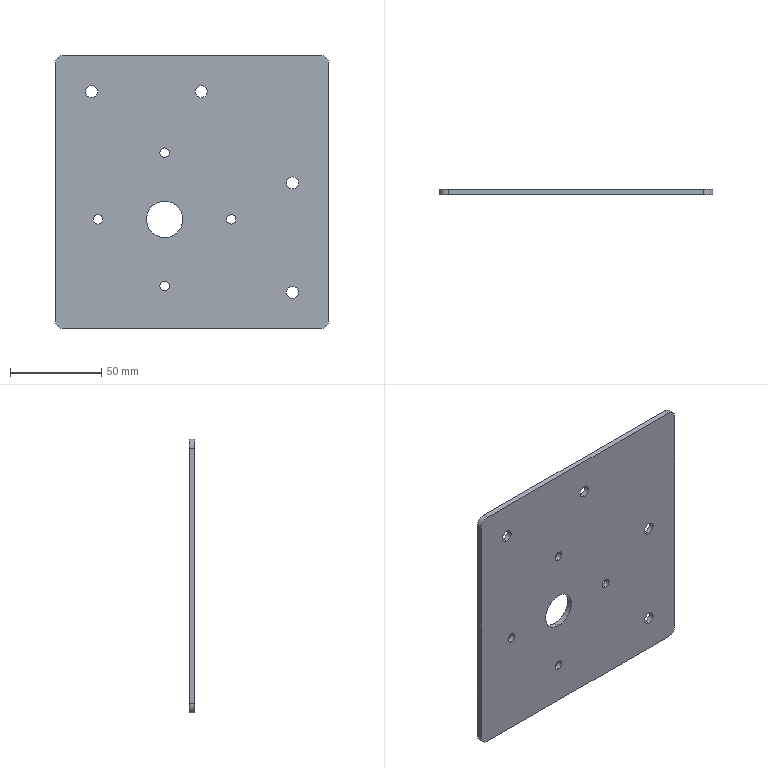Part | SolidWorks | features Extrusion 1, Fillet 1, HoleWzd 1, ICE 1 | 1 solid | 28 faces | box 150 x 3 x 150 mm | volume 65828 mm3 | cylinder 22 | plane 6 | commonest cylinder face diameters 5.2 x8 6.6 x8 10 x4 20 x2
STEP:
#1=CARTESIAN_POINT('',(-51.5,0.,-17.6));
#2=VERTEX_POINT('',#1);
#3=CARTESIAN_POINT('',(-51.5,0.,-12.4));
#4=VERTEX_POINT('',#3);
#5=CARTESIAN_POINT('',(-51.5,0.,-15.));
#6=DIRECTION('',(0.,1.,0.));
#7=DIRECTION('',(0.,0.,1.));
#8=AXIS2_PLACEMENT_3D('',#5,#6,#7);
#9=CIRCLE('',#8,2.6);
#10=EDGE_CURVE('',#2,#4,#9,.T.);
#11=ORIENTED_EDGE('',*,*,#10,.F.);
#12=CARTESIAN_POINT('',(-51.5,3.,-17.6));
#13=VERTEX_POINT('',#12);
#14=CARTESIAN_POINT('',(-51.5,0.,-17.6));
#15=DIRECTION('',(0.,1.,0.));
#16=VECTOR('',#15,1000.);
#17=LINE('',#14,#16);
#18=EDGE_CURVE('',#2,#13,#17,.T.);
#19=ORIENTED_EDGE('',*,*,#18,.T.);
#20=CARTESIAN_POINT('',(-51.5,3.,-12.4));
#21=VERTEX_POINT('',#20);
#22=CARTESIAN_POINT('',(-51.5,3.,-15.));
#23=DIRECTION('',(0.,1.,0.));
#24=DIRECTION('',(0.,0.,1.));
#25=AXIS2_PLACEMENT_3D('',#22,#23,#24);
#26=CIRCLE('',#25,2.6);
#27=EDGE_CURVE('',#13,#21,#26,.T.);
#28=ORIENTED_EDGE('',*,*,#27,.T.);
#29=CARTESIAN_POINT('',(-51.5,0.,-12.4));
#30=DIRECTION('',(0.,1.,0.));
#31=VECTOR('',#30,1000.);
#32=LINE('',#29,#31);
#33=EDGE_CURVE('',#4,#21,#32,.T.);
#34=ORIENTED_EDGE('',*,*,#33,.F.);
#35=EDGE_LOOP('',(#11,#19,#28,#34));
#36=FACE_OUTER_BOUND('',#35,.T.);
#37=CARTESIAN_POINT('',(-51.5,0.,-15.));
#38=DIRECTION('',(0.,1.,0.));
#39=DIRECTION('',(0.,0.,1.));
#40=AXIS2_PLACEMENT_3D('',#37,#38,#39);
#41=CYLINDRICAL_SURFACE('',#40,2.6);
#42=ADVANCED_FACE('',(#36),#41,.F.);
#43=CARTESIAN_POINT('',(-15.,0.,18.9));
#44=VERTEX_POINT('',#43);
#45=CARTESIAN_POINT('',(-15.,0.,24.1));
#46=VERTEX_POINT('',#45);
#47=CARTESIAN_POINT('',(-15.,0.,21.5));
#48=DIRECTION('',(0.,1.,0.));
#49=DIRECTION('',(0.,0.,1.));
#50=AXIS2_PLACEMENT_3D('',#47,#48,#49);
#51=CIRCLE('',#50,2.6);
#52=EDGE_CURVE('',#44,#46,#51,.T.);
#53=ORIENTED_EDGE('',*,*,#52,.F.);
#54=CARTESIAN_POINT('',(-15.,3.,18.9));
#55=VERTEX_POINT('',#54);
#56=CARTESIAN_POINT('',(-15.,0.,18.9));
#57=DIRECTION('',(0.,1.,0.));
#58=VECTOR('',#57,1000.);
#59=LINE('',#56,#58);
#60=EDGE_CURVE('',#44,#55,#59,.T.);
#61=ORIENTED_EDGE('',*,*,#60,.T.);
#62=CARTESIAN_POINT('',(-15.,3.,24.1));
#63=VERTEX_POINT('',#62);
#64=CARTESIAN_POINT('',(-15.,3.,21.5));
#65=DIRECTION('',(0.,1.,0.));
#66=DIRECTION('',(0.,0.,1.));
#67=AXIS2_PLACEMENT_3D('',#64,#65,#66);
#68=CIRCLE('',#67,2.6);
#69=EDGE_CURVE('',#55,#63,#68,.T.);
#70=ORIENTED_EDGE('',*,*,#69,.T.);
#71=CARTESIAN_POINT('',(-15.,0.,24.1));
#72=DIRECTION('',(0.,1.,0.));
#73=VECTOR('',#72,1000.);
#74=LINE('',#71,#73);
#75=EDGE_CURVE('',#46,#63,#74,.T.);
#76=ORIENTED_EDGE('',*,*,#75,.F.);
#77=EDGE_LOOP('',(#53,#61,#70,#76));
#78=FACE_OUTER_BOUND('',#77,.T.);
#79=CARTESIAN_POINT('',(-15.,0.,21.5));
#80=DIRECTION('',(0.,1.,0.));
#81=DIRECTION('',(0.,0.,1.));
#82=AXIS2_PLACEMENT_3D('',#79,#80,#81);
#83=CYLINDRICAL_SURFACE('',#82,2.6);
#84=ADVANCED_FACE('',(#78),#83,.F.);
#85=CARTESIAN_POINT('',(21.5,0.,-17.6));
#86=VERTEX_POINT('',#85);
#87=CARTESIAN_POINT('',(21.5,0.,-12.4));
#88=VERTEX_POINT('',#87);
#89=CARTESIAN_POINT('',(21.5,0.,-15.));
#90=DIRECTION('',(0.,1.,0.));
#91=DIRECTION('',(0.,0.,1.));
#92=AXIS2_PLACEMENT_3D('',#89,#90,#91);
#93=CIRCLE('',#92,2.6);
#94=EDGE_CURVE('',#86,#88,#93,.T.);
#95=ORIENTED_EDGE('',*,*,#94,.F.);
#96=CARTESIAN_POINT('',(21.5,3.,-17.6));
#97=VERTEX_POINT('',#96);
#98=CARTESIAN_POINT('',(21.5,0.,-17.6));
#99=DIRECTION('',(0.,1.,0.));
#100=VECTOR('',#99,1000.);
#101=LINE('',#98,#100);
#102=EDGE_CURVE('',#86,#97,#101,.T.);
#103=ORIENTED_EDGE('',*,*,#102,.T.);
#104=CARTESIAN_POINT('',(21.5,3.,-12.4));
#105=VERTEX_POINT('',#104);
#106=CARTESIAN_POINT('',(21.5,3.,-15.));
#107=DIRECTION('',(0.,1.,0.));
#108=DIRECTION('',(0.,0.,1.));
#109=AXIS2_PLACEMENT_3D('',#106,#107,#108);
#110=CIRCLE('',#109,2.6);
#111=EDGE_CURVE('',#97,#105,#110,.T.);
#112=ORIENTED_EDGE('',*,*,#111,.T.);
#113=CARTESIAN_POINT('',(21.5,0.,-12.4));
#114=DIRECTION('',(0.,1.,0.));
#115=VECTOR('',#114,1000.);
#116=LINE('',#113,#115);
#117=EDGE_CURVE('',#88,#105,#116,.T.);
#118=ORIENTED_EDGE('',*,*,#117,.F.);
#119=EDGE_LOOP('',(#95,#103,#112,#118));
#120=FACE_OUTER_BOUND('',#119,.T.);
#121=CARTESIAN_POINT('',(21.5,0.,-15.));
#122=DIRECTION('',(0.,1.,0.));
#123=DIRECTION('',(0.,0.,1.));
#124=AXIS2_PLACEMENT_3D('',#121,#122,#123);
#125=CYLINDRICAL_SURFACE('',#124,2.6);
#126=ADVANCED_FACE('',(#120),#125,.F.);
#127=CARTESIAN_POINT('',(-15.,0.,-54.1));
#128=VERTEX_POINT('',#127);
#129=CARTESIAN_POINT('',(-15.,0.,-48.9));
#130=VERTEX_POINT('',#129);
#131=CARTESIAN_POINT('',(-15.,0.,-51.5));
#132=DIRECTION('',(0.,1.,0.));
#133=DIRECTION('',(0.,0.,1.));
#134=AXIS2_PLACEMENT_3D('',#131,#132,#133);
#135=CIRCLE('',#134,2.6);
#136=EDGE_CURVE('',#128,#130,#135,.T.);
#137=ORIENTED_EDGE('',*,*,#136,.F.);
#138=CARTESIAN_POINT('',(-15.,3.,-54.1));
#139=VERTEX_POINT('',#138);
#140=CARTESIAN_POINT('',(-15.,0.,-54.1));
#141=DIRECTION('',(0.,1.,0.));
#142=VECTOR('',#141,1000.);
#143=LINE('',#140,#142);
#144=EDGE_CURVE('',#128,#139,#143,.T.);
#145=ORIENTED_EDGE('',*,*,#144,.T.);
#146=CARTESIAN_POINT('',(-15.,3.,-48.9));
#147=VERTEX_POINT('',#146);
#148=CARTESIAN_POINT('',(-15.,3.,-51.5));
#149=DIRECTION('',(0.,1.,0.));
#150=DIRECTION('',(0.,0.,1.));
#151=AXIS2_PLACEMENT_3D('',#148,#149,#150);
#152=CIRCLE('',#151,2.6);
#153=EDGE_CURVE('',#139,#147,#152,.T.);
#154=ORIENTED_EDGE('',*,*,#153,.T.);
#155=CARTESIAN_POINT('',(-15.,0.,-48.9));
#156=DIRECTION('',(0.,1.,0.));
#157=VECTOR('',#156,1000.);
#158=LINE('',#155,#157);
#159=EDGE_CURVE('',#130,#147,#158,.T.);
#160=ORIENTED_EDGE('',*,*,#159,.F.);
#161=EDGE_LOOP('',(#137,#145,#154,#160));
#162=FACE_OUTER_BOUND('',#161,.T.);
#163=CARTESIAN_POINT('',(-15.,0.,-51.5));
#164=DIRECTION('',(0.,1.,0.));
#165=DIRECTION('',(0.,0.,1.));
#166=AXIS2_PLACEMENT_3D('',#163,#164,#165);
#167=CYLINDRICAL_SURFACE('',#166,2.6);
#168=ADVANCED_FACE('',(#162),#167,.F.);
#169=CARTESIAN_POINT('',(-15.,0.,-25.));
#170=VERTEX_POINT('',#169);
#171=CARTESIAN_POINT('',(-15.,0.,-5.));
#172=VERTEX_POINT('',#171);
#173=CARTESIAN_POINT('',(-15.,0.,-15.));
#174=DIRECTION('',(0.,1.,0.));
#175=DIRECTION('',(0.,0.,1.));
#176=AXIS2_PLACEMENT_3D('',#173,#174,#175);
#177=CIRCLE('',#176,10.);
#178=EDGE_CURVE('',#170,#172,#177,.T.);
#179=ORIENTED_EDGE('',*,*,#178,.F.);
#180=CARTESIAN_POINT('',(-15.,3.,-25.));
#181=VERTEX_POINT('',#180);
#182=CARTESIAN_POINT('',(-15.,0.,-25.));
#183=DIRECTION('',(0.,1.,0.));
#184=VECTOR('',#183,1000.);
#185=LINE('',#182,#184);
#186=EDGE_CURVE('',#170,#181,#185,.T.);
#187=ORIENTED_EDGE('',*,*,#186,.T.);
#188=CARTESIAN_POINT('',(-15.,3.,-5.));
#189=VERTEX_POINT('',#188);
#190=CARTESIAN_POINT('',(-15.,3.,-15.));
#191=DIRECTION('',(0.,1.,0.));
#192=DIRECTION('',(0.,0.,1.));
#193=AXIS2_PLACEMENT_3D('',#190,#191,#192);
#194=CIRCLE('',#193,10.);
#195=EDGE_CURVE('',#181,#189,#194,.T.);
#196=ORIENTED_EDGE('',*,*,#195,.T.);
#197=CARTESIAN_POINT('',(-15.,0.,-5.));
#198=DIRECTION('',(0.,1.,0.));
#199=VECTOR('',#198,1000.);
#200=LINE('',#197,#199);
#201=EDGE_CURVE('',#172,#189,#200,.T.);
#202=ORIENTED_EDGE('',*,*,#201,.F.);
#203=EDGE_LOOP('',(#179,#187,#196,#202));
#204=FACE_OUTER_BOUND('',#203,.T.);
#205=CARTESIAN_POINT('',(-15.,0.,-15.));
#206=DIRECTION('',(0.,1.,0.));
#207=DIRECTION('',(0.,0.,1.));
#208=AXIS2_PLACEMENT_3D('',#205,#206,#207);
#209=CYLINDRICAL_SURFACE('',#208,10.);
#210=ADVANCED_FACE('',(#204),#209,.F.);
#211=CARTESIAN_POINT('',(55.,0.,1.7));
#212=VERTEX_POINT('',#211);
#213=CARTESIAN_POINT('',(55.,0.,8.3));
#214=VERTEX_POINT('',#213);
#215=CARTESIAN_POINT('',(55.,0.,5.));
#216=DIRECTION('',(0.,1.,0.));
#217=DIRECTION('',(0.,0.,1.));
#218=AXIS2_PLACEMENT_3D('',#215,#216,#217);
#219=CIRCLE('',#218,3.3);
#220=EDGE_CURVE('',#212,#214,#219,.T.);
#221=ORIENTED_EDGE('',*,*,#220,.F.);
#222=CARTESIAN_POINT('',(55.,3.,1.7));
#223=VERTEX_POINT('',#222);
#224=CARTESIAN_POINT('',(55.,3.,1.7));
#225=DIRECTION('',(0.,1.,0.));
#226=VECTOR('',#225,1000.);
#227=LINE('',#224,#226);
#228=EDGE_CURVE('',#212,#223,#227,.T.);
#229=ORIENTED_EDGE('',*,*,#228,.T.);
#230=CARTESIAN_POINT('',(55.,3.,8.3));
#231=VERTEX_POINT('',#230);
#232=CARTESIAN_POINT('',(55.,3.,5.));
#233=DIRECTION('',(0.,1.,0.));
#234=DIRECTION('',(0.,0.,1.));
#235=AXIS2_PLACEMENT_3D('',#232,#233,#234);
#236=CIRCLE('',#235,3.3);
#237=EDGE_CURVE('',#223,#231,#236,.T.);
#238=ORIENTED_EDGE('',*,*,#237,.T.);
#239=CARTESIAN_POINT('',(55.,3.,8.3));
#240=DIRECTION('',(0.,1.,0.));
#241=VECTOR('',#240,1000.);
#242=LINE('',#239,#241);
#243=EDGE_CURVE('',#214,#231,#242,.T.);
#244=ORIENTED_EDGE('',*,*,#243,.F.);
#245=EDGE_LOOP('',(#221,#229,#238,#244));
#246=FACE_OUTER_BOUND('',#245,.T.);
#247=CARTESIAN_POINT('',(55.,3.,5.));
#248=DIRECTION('',(0.,1.,0.));
#249=DIRECTION('',(0.,0.,1.));
#250=AXIS2_PLACEMENT_3D('',#247,#248,#249);
#251=CYLINDRICAL_SURFACE('',#250,3.3);
#252=ADVANCED_FACE('',(#246),#251,.F.);
#253=CARTESIAN_POINT('',(5.,0.,51.7));
#254=VERTEX_POINT('',#253);
#255=CARTESIAN_POINT('',(5.,0.,58.3));
#256=VERTEX_POINT('',#255);
#257=CARTESIAN_POINT('',(5.,0.,55.));
#258=DIRECTION('',(0.,1.,0.));
#259=DIRECTION('',(0.,0.,1.));
#260=AXIS2_PLACEMENT_3D('',#257,#258,#259);
#261=CIRCLE('',#260,3.3);
#262=EDGE_CURVE('',#254,#256,#261,.T.);
#263=ORIENTED_EDGE('',*,*,#262,.F.);
#264=CARTESIAN_POINT('',(5.,3.,51.7));
#265=VERTEX_POINT('',#264);
#266=CARTESIAN_POINT('',(5.,3.,51.7));
#267=DIRECTION('',(0.,1.,0.));
#268=VECTOR('',#267,1000.);
#269=LINE('',#266,#268);
#270=EDGE_CURVE('',#254,#265,#269,.T.);
#271=ORIENTED_EDGE('',*,*,#270,.T.);
#272=CARTESIAN_POINT('',(5.,3.,58.3));
#273=VERTEX_POINT('',#272);
#274=CARTESIAN_POINT('',(5.,3.,55.));
#275=DIRECTION('',(0.,1.,0.));
#276=DIRECTION('',(0.,0.,1.));
#277=AXIS2_PLACEMENT_3D('',#274,#275,#276);
#278=CIRCLE('',#277,3.3);
#279=EDGE_CURVE('',#265,#273,#278,.T.);
#280=ORIENTED_EDGE('',*,*,#279,.T.);
#281=CARTESIAN_POINT('',(5.,3.,58.3));
#282=DIRECTION('',(0.,1.,0.));
#283=VECTOR('',#282,1000.);
#284=LINE('',#281,#283);
#285=EDGE_CURVE('',#256,#273,#284,.T.);
#286=ORIENTED_EDGE('',*,*,#285,.F.);
#287=EDGE_LOOP('',(#263,#271,#280,#286));
#288=FACE_OUTER_BOUND('',#287,.T.);
#289=CARTESIAN_POINT('',(5.,3.,55.));
#290=DIRECTION('',(0.,1.,0.));
#291=DIRECTION('',(0.,0.,1.));
#292=AXIS2_PLACEMENT_3D('',#289,#290,#291);
#293=CYLINDRICAL_SURFACE('',#292,3.3);
#294=ADVANCED_FACE('',(#288),#293,.F.);
#295=CARTESIAN_POINT('',(-55.,0.,51.7));
#296=VERTEX_POINT('',#295);
#297=CARTESIAN_POINT('',(-55.,0.,58.3));
#298=VERTEX_POINT('',#297);
#299=CARTESIAN_POINT('',(-55.,0.,55.));
#300=DIRECTION('',(0.,1.,0.));
#301=DIRECTION('',(0.,0.,1.));
#302=AXIS2_PLACEMENT_3D('',#299,#300,#301);
#303=CIRCLE('',#302,3.3);
#304=EDGE_CURVE('',#296,#298,#303,.T.);
#305=ORIENTED_EDGE('',*,*,#304,.F.);
#306=CARTESIAN_POINT('',(-55.,3.,51.7));
#307=VERTEX_POINT('',#306);
#308=CARTESIAN_POINT('',(-55.,3.,51.7));
#309=DIRECTION('',(0.,1.,0.));
#310=VECTOR('',#309,1000.);
#311=LINE('',#308,#310);
#312=EDGE_CURVE('',#296,#307,#311,.T.);
#313=ORIENTED_EDGE('',*,*,#312,.T.);
#314=CARTESIAN_POINT('',(-55.,3.,58.3));
#315=VERTEX_POINT('',#314);
#316=CARTESIAN_POINT('',(-55.,3.,55.));
#317=DIRECTION('',(0.,1.,0.));
#318=DIRECTION('',(0.,0.,1.));
#319=AXIS2_PLACEMENT_3D('',#316,#317,#318);
#320=CIRCLE('',#319,3.3);
#321=EDGE_CURVE('',#307,#315,#320,.T.);
#322=ORIENTED_EDGE('',*,*,#321,.T.);
#323=CARTESIAN_POINT('',(-55.,3.,58.3));
#324=DIRECTION('',(0.,1.,0.));
#325=VECTOR('',#324,1000.);
#326=LINE('',#323,#325);
#327=EDGE_CURVE('',#298,#315,#326,.T.);
#328=ORIENTED_EDGE('',*,*,#327,.F.);
#329=EDGE_LOOP('',(#305,#313,#322,#328));
#330=FACE_OUTER_BOUND('',#329,.T.);
#331=CARTESIAN_POINT('',(-55.,3.,55.));
#332=DIRECTION('',(0.,1.,0.));
#333=DIRECTION('',(0.,0.,1.));
#334=AXIS2_PLACEMENT_3D('',#331,#332,#333);
#335=CYLINDRICAL_SURFACE('',#334,3.3);
#336=ADVANCED_FACE('',(#330),#335,.F.);
#337=CARTESIAN_POINT('',(55.,0.,-58.3));
#338=VERTEX_POINT('',#337);
#339=CARTESIAN_POINT('',(55.,0.,-51.7));
#340=VERTEX_POINT('',#339);
#341=CARTESIAN_POINT('',(55.,0.,-55.));
#342=DIRECTION('',(0.,1.,0.));
#343=DIRECTION('',(0.,0.,1.));
#344=AXIS2_PLACEMENT_3D('',#341,#342,#343);
#345=CIRCLE('',#344,3.3);
#346=EDGE_CURVE('',#338,#340,#345,.T.);
#347=ORIENTED_EDGE('',*,*,#346,.F.);
#348=CARTESIAN_POINT('',(55.,3.,-58.3));
#349=VERTEX_POINT('',#348);
#350=CARTESIAN_POINT('',(55.,3.,-58.3));
#351=DIRECTION('',(0.,1.,0.));
#352=VECTOR('',#351,1000.);
#353=LINE('',#350,#352);
#354=EDGE_CURVE('',#338,#349,#353,.T.);
#355=ORIENTED_EDGE('',*,*,#354,.T.);
#356=CARTESIAN_POINT('',(55.,3.,-51.7));
#357=VERTEX_POINT('',#356);
#358=CARTESIAN_POINT('',(55.,3.,-55.));
#359=DIRECTION('',(0.,1.,0.));
#360=DIRECTION('',(0.,0.,1.));
#361=AXIS2_PLACEMENT_3D('',#358,#359,#360);
#362=CIRCLE('',#361,3.3);
#363=EDGE_CURVE('',#349,#357,#362,.T.);
#364=ORIENTED_EDGE('',*,*,#363,.T.);
#365=CARTESIAN_POINT('',(55.,3.,-51.7));
#366=DIRECTION('',(0.,1.,0.));
#367=VECTOR('',#366,1000.);
#368=LINE('',#365,#367);
#369=EDGE_CURVE('',#340,#357,#368,.T.);
#370=ORIENTED_EDGE('',*,*,#369,.F.);
#371=EDGE_LOOP('',(#347,#355,#364,#370));
#372=FACE_OUTER_BOUND('',#371,.T.);
#373=CARTESIAN_POINT('',(55.,3.,-55.));
#374=DIRECTION('',(0.,1.,0.));
#375=DIRECTION('',(0.,0.,1.));
#376=AXIS2_PLACEMENT_3D('',#373,#374,#375);
#377=CYLINDRICAL_SURFACE('',#376,3.3);
#378=ADVANCED_FACE('',(#372),#377,.F.);
#379=CARTESIAN_POINT('',(75.,0.,70.));
#380=VERTEX_POINT('',#379);
#381=CARTESIAN_POINT('',(75.,0.,-70.));
#382=VERTEX_POINT('',#381);
#383=CARTESIAN_POINT('',(75.,0.,-75.));
#384=DIRECTION('',(0.,0.,-1.));
#385=VECTOR('',#384,1000.);
#386=LINE('',#383,#385);
#387=EDGE_CURVE('',#380,#382,#386,.T.);
#388=ORIENTED_EDGE('',*,*,#387,.T.);
#389=CARTESIAN_POINT('',(75.,3.,-70.));
#390=VERTEX_POINT('',#389);
#391=CARTESIAN_POINT('',(75.,3.,-70.));
#392=DIRECTION('',(0.,1.,0.));
#393=VECTOR('',#392,1000.);
#394=LINE('',#391,#393);
#395=EDGE_CURVE('',#382,#390,#394,.T.);
#396=ORIENTED_EDGE('',*,*,#395,.T.);
#397=CARTESIAN_POINT('',(75.,3.,70.));
#398=VERTEX_POINT('',#397);
#399=CARTESIAN_POINT('',(75.,3.,-75.));
#400=DIRECTION('',(0.,0.,-1.));
#401=VECTOR('',#400,1000.);
#402=LINE('',#399,#401);
#403=EDGE_CURVE('',#398,#390,#402,.T.);
#404=ORIENTED_EDGE('',*,*,#403,.F.);
#405=CARTESIAN_POINT('',(75.,3.,70.));
#406=DIRECTION('',(0.,-1.,0.));
#407=VECTOR('',#406,1000.);
#408=LINE('',#405,#407);
#409=EDGE_CURVE('',#398,#380,#408,.T.);
#410=ORIENTED_EDGE('',*,*,#409,.T.);
#411=EDGE_LOOP('',(#388,#396,#404,#410));
#412=FACE_OUTER_BOUND('',#411,.T.);
#413=CARTESIAN_POINT('',(75.,3.,-75.));
#414=DIRECTION('',(-1.,0.,0.));
#415=DIRECTION('',(0.,0.,1.));
#416=AXIS2_PLACEMENT_3D('',#413,#414,#415);
#417=PLANE('',#416);
#418=ADVANCED_FACE('',(#412),#417,.F.);
#419=CARTESIAN_POINT('',(70.,0.,-75.));
#420=VERTEX_POINT('',#419);
#421=CARTESIAN_POINT('',(-70.,0.,-75.));
#422=VERTEX_POINT('',#421);
#423=CARTESIAN_POINT('',(-75.,0.,-75.));
#424=DIRECTION('',(-1.,0.,0.));
#425=VECTOR('',#424,1000.);
#426=LINE('',#423,#425);
#427=EDGE_CURVE('',#420,#422,#426,.T.);
#428=ORIENTED_EDGE('',*,*,#427,.T.);
#429=CARTESIAN_POINT('',(-70.,3.,-75.));
#430=VERTEX_POINT('',#429);
#431=CARTESIAN_POINT('',(-70.,3.,-75.));
#432=DIRECTION('',(0.,1.,0.));
#433=VECTOR('',#432,1000.);
#434=LINE('',#431,#433);
#435=EDGE_CURVE('',#422,#430,#434,.T.);
#436=ORIENTED_EDGE('',*,*,#435,.T.);
#437=CARTESIAN_POINT('',(70.,3.,-75.));
#438=VERTEX_POINT('',#437);
#439=CARTESIAN_POINT('',(-75.,3.,-75.));
#440=DIRECTION('',(-1.,0.,0.));
#441=VECTOR('',#440,1000.);
#442=LINE('',#439,#441);
#443=EDGE_CURVE('',#438,#430,#442,.T.);
#444=ORIENTED_EDGE('',*,*,#443,.F.);
#445=CARTESIAN_POINT('',(70.,3.,-75.));
#446=DIRECTION('',(0.,-1.,0.));
#447=VECTOR('',#446,1000.);
#448=LINE('',#445,#447);
#449=EDGE_CURVE('',#438,#420,#448,.T.);
#450=ORIENTED_EDGE('',*,*,#449,.T.);
#451=EDGE_LOOP('',(#428,#436,#444,#450));
#452=FACE_OUTER_BOUND('',#451,.T.);
#453=CARTESIAN_POINT('',(-75.,3.,-75.));
#454=DIRECTION('',(0.,0.,1.));
#455=DIRECTION('',(1.,0.,0.));
#456=AXIS2_PLACEMENT_3D('',#453,#454,#455);
#457=PLANE('',#456);
#458=ADVANCED_FACE('',(#452),#457,.F.);
#459=CARTESIAN_POINT('',(-75.,0.,-70.));
#460=VERTEX_POINT('',#459);
#461=CARTESIAN_POINT('',(-75.,0.,70.));
#462=VERTEX_POINT('',#461);
#463=CARTESIAN_POINT('',(-75.,0.,-75.));
#464=DIRECTION('',(0.,0.,1.));
#465=VECTOR('',#464,1000.);
#466=LINE('',#463,#465);
#467=EDGE_CURVE('',#460,#462,#466,.T.);
#468=ORIENTED_EDGE('',*,*,#467,.T.);
#469=CARTESIAN_POINT('',(-75.,3.,70.));
#470=VERTEX_POINT('',#469);
#471=CARTESIAN_POINT('',(-75.,3.,70.));
#472=DIRECTION('',(0.,1.,0.));
#473=VECTOR('',#472,1000.);
#474=LINE('',#471,#473);
#475=EDGE_CURVE('',#462,#470,#474,.T.);
#476=ORIENTED_EDGE('',*,*,#475,.T.);
#477=CARTESIAN_POINT('',(-75.,3.,-70.));
#478=VERTEX_POINT('',#477);
#479=CARTESIAN_POINT('',(-75.,3.,-75.));
#480=DIRECTION('',(0.,0.,1.));
#481=VECTOR('',#480,1000.);
#482=LINE('',#479,#481);
#483=EDGE_CURVE('',#478,#470,#482,.T.);
#484=ORIENTED_EDGE('',*,*,#483,.F.);
#485=CARTESIAN_POINT('',(-75.,3.,-70.));
#486=DIRECTION('',(0.,-1.,0.));
#487=VECTOR('',#486,1000.);
#488=LINE('',#485,#487);
#489=EDGE_CURVE('',#478,#460,#488,.T.);
#490=ORIENTED_EDGE('',*,*,#489,.T.);
#491=EDGE_LOOP('',(#468,#476,#484,#490));
#492=FACE_OUTER_BOUND('',#491,.T.);
#493=CARTESIAN_POINT('',(-75.,3.,-75.));
#494=DIRECTION('',(1.,0.,0.));
#495=DIRECTION('',(0.,0.,-1.));
#496=AXIS2_PLACEMENT_3D('',#493,#494,#495);
#497=PLANE('',#496);
#498=ADVANCED_FACE('',(#492),#497,.F.);
#499=CARTESIAN_POINT('',(-70.,3.,75.));
#500=VERTEX_POINT('',#499);
#501=CARTESIAN_POINT('',(70.,3.,75.));
#502=VERTEX_POINT('',#501);
#503=CARTESIAN_POINT('',(-75.,3.,75.));
#504=DIRECTION('',(1.,0.,0.));
#505=VECTOR('',#504,1000.);
#506=LINE('',#503,#505);
#507=EDGE_CURVE('',#500,#502,#506,.T.);
#508=ORIENTED_EDGE('',*,*,#507,.F.);
#509=CARTESIAN_POINT('',(-70.,0.,75.));
#510=VERTEX_POINT('',#509);
#511=CARTESIAN_POINT('',(-70.,3.,75.));
#512=DIRECTION('',(0.,-1.,0.));
#513=VECTOR('',#512,1000.);
#514=LINE('',#511,#513);
#515=EDGE_CURVE('',#500,#510,#514,.T.);
#516=ORIENTED_EDGE('',*,*,#515,.T.);
#517=CARTESIAN_POINT('',(70.,0.,75.));
#518=VERTEX_POINT('',#517);
#519=CARTESIAN_POINT('',(-75.,0.,75.));
#520=DIRECTION('',(1.,0.,0.));
#521=VECTOR('',#520,1000.);
#522=LINE('',#519,#521);
#523=EDGE_CURVE('',#510,#518,#522,.T.);
#524=ORIENTED_EDGE('',*,*,#523,.T.);
#525=CARTESIAN_POINT('',(70.,3.,75.));
#526=DIRECTION('',(0.,1.,0.));
#527=VECTOR('',#526,1000.);
#528=LINE('',#525,#527);
#529=EDGE_CURVE('',#518,#502,#528,.T.);
#530=ORIENTED_EDGE('',*,*,#529,.T.);
#531=EDGE_LOOP('',(#508,#516,#524,#530));
#532=FACE_OUTER_BOUND('',#531,.T.);
#533=CARTESIAN_POINT('',(-75.,3.,75.));
#534=DIRECTION('',(0.,0.,-1.));
#535=DIRECTION('',(-1.,0.,0.));
#536=AXIS2_PLACEMENT_3D('',#533,#534,#535);
#537=PLANE('',#536);
#538=ADVANCED_FACE('',(#532),#537,.F.);
#539=CARTESIAN_POINT('',(-51.5,3.,-15.));
#540=DIRECTION('',(0.,1.,0.));
#541=DIRECTION('',(0.,0.,1.));
#542=AXIS2_PLACEMENT_3D('',#539,#540,#541);
#543=CIRCLE('',#542,2.6);
#544=EDGE_CURVE('',#21,#13,#543,.T.);
#545=ORIENTED_EDGE('',*,*,#544,.F.);
#546=ORIENTED_EDGE('',*,*,#27,.F.);
#547=EDGE_LOOP('',(#545,#546));
#548=FACE_BOUND('',#547,.T.);
#549=CARTESIAN_POINT('',(-15.,3.,21.5));
#550=DIRECTION('',(0.,1.,0.));
#551=DIRECTION('',(0.,0.,1.));
#552=AXIS2_PLACEMENT_3D('',#549,#550,#551);
#553=CIRCLE('',#552,2.6);
#554=EDGE_CURVE('',#63,#55,#553,.T.);
#555=ORIENTED_EDGE('',*,*,#554,.F.);
#556=ORIENTED_EDGE('',*,*,#69,.F.);
#557=EDGE_LOOP('',(#555,#556));
#558=FACE_BOUND('',#557,.T.);
#559=CARTESIAN_POINT('',(21.5,3.,-15.));
#560=DIRECTION('',(0.,1.,0.));
#561=DIRECTION('',(0.,0.,1.));
#562=AXIS2_PLACEMENT_3D('',#559,#560,#561);
#563=CIRCLE('',#562,2.6);
#564=EDGE_CURVE('',#105,#97,#563,.T.);
#565=ORIENTED_EDGE('',*,*,#564,.F.);
#566=ORIENTED_EDGE('',*,*,#111,.F.);
#567=EDGE_LOOP('',(#565,#566));
#568=FACE_BOUND('',#567,.T.);
#569=CARTESIAN_POINT('',(-15.,3.,-51.5));
#570=DIRECTION('',(0.,1.,0.));
#571=DIRECTION('',(0.,0.,1.));
#572=AXIS2_PLACEMENT_3D('',#569,#570,#571);
#573=CIRCLE('',#572,2.6);
#574=EDGE_CURVE('',#147,#139,#573,.T.);
#575=ORIENTED_EDGE('',*,*,#574,.F.);
#576=ORIENTED_EDGE('',*,*,#153,.F.);
#577=EDGE_LOOP('',(#575,#576));
#578=FACE_BOUND('',#577,.T.);
#579=CARTESIAN_POINT('',(-15.,3.,-15.));
#580=DIRECTION('',(0.,1.,0.));
#581=DIRECTION('',(0.,0.,1.));
#582=AXIS2_PLACEMENT_3D('',#579,#580,#581);
#583=CIRCLE('',#582,10.);
#584=EDGE_CURVE('',#189,#181,#583,.T.);
#585=ORIENTED_EDGE('',*,*,#584,.F.);
#586=ORIENTED_EDGE('',*,*,#195,.F.);
#587=EDGE_LOOP('',(#585,#586));
#588=FACE_BOUND('',#587,.T.);
#589=CARTESIAN_POINT('',(55.,3.,5.));
#590=DIRECTION('',(0.,1.,0.));
#591=DIRECTION('',(0.,0.,1.));
#592=AXIS2_PLACEMENT_3D('',#589,#590,#591);
#593=CIRCLE('',#592,3.3);
#594=EDGE_CURVE('',#231,#223,#593,.T.);
#595=ORIENTED_EDGE('',*,*,#594,.F.);
#596=ORIENTED_EDGE('',*,*,#237,.F.);
#597=EDGE_LOOP('',(#595,#596));
#598=FACE_BOUND('',#597,.T.);
#599=CARTESIAN_POINT('',(5.,3.,55.));
#600=DIRECTION('',(0.,1.,0.));
#601=DIRECTION('',(0.,0.,1.));
#602=AXIS2_PLACEMENT_3D('',#599,#600,#601);
#603=CIRCLE('',#602,3.3);
#604=EDGE_CURVE('',#273,#265,#603,.T.);
#605=ORIENTED_EDGE('',*,*,#604,.F.);
#606=ORIENTED_EDGE('',*,*,#279,.F.);
#607=EDGE_LOOP('',(#605,#606));
#608=FACE_BOUND('',#607,.T.);
#609=CARTESIAN_POINT('',(-55.,3.,55.));
#610=DIRECTION('',(0.,1.,0.));
#611=DIRECTION('',(0.,0.,1.));
#612=AXIS2_PLACEMENT_3D('',#609,#610,#611);
#613=CIRCLE('',#612,3.3);
#614=EDGE_CURVE('',#315,#307,#613,.T.);
#615=ORIENTED_EDGE('',*,*,#614,.F.);
#616=ORIENTED_EDGE('',*,*,#321,.F.);
#617=EDGE_LOOP('',(#615,#616));
#618=FACE_BOUND('',#617,.T.);
#619=CARTESIAN_POINT('',(55.,3.,-55.));
#620=DIRECTION('',(0.,1.,0.));
#621=DIRECTION('',(0.,0.,1.));
#622=AXIS2_PLACEMENT_3D('',#619,#620,#621);
#623=CIRCLE('',#622,3.3);
#624=EDGE_CURVE('',#357,#349,#623,.T.);
#625=ORIENTED_EDGE('',*,*,#624,.F.);
#626=ORIENTED_EDGE('',*,*,#363,.F.);
#627=EDGE_LOOP('',(#625,#626));
#628=FACE_BOUND('',#627,.T.);
#629=ORIENTED_EDGE('',*,*,#483,.T.);
#630=CARTESIAN_POINT('',(-70.,3.,70.));
#631=DIRECTION('',(0.,1.,0.));
#632=DIRECTION('',(0.,0.,1.));
#633=AXIS2_PLACEMENT_3D('',#630,#631,#632);
#634=CIRCLE('',#633,5.);
#635=EDGE_CURVE('',#470,#500,#634,.T.);
#636=ORIENTED_EDGE('',*,*,#635,.T.);
#637=ORIENTED_EDGE('',*,*,#507,.T.);
#638=CARTESIAN_POINT('',(70.,3.,70.));
#639=DIRECTION('',(0.,1.,0.));
#640=DIRECTION('',(0.,0.,1.));
#641=AXIS2_PLACEMENT_3D('',#638,#639,#640);
#642=CIRCLE('',#641,5.);
#643=EDGE_CURVE('',#502,#398,#642,.T.);
#644=ORIENTED_EDGE('',*,*,#643,.T.);
#645=ORIENTED_EDGE('',*,*,#403,.T.);
#646=CARTESIAN_POINT('',(70.,3.,-70.));
#647=DIRECTION('',(0.,1.,0.));
#648=DIRECTION('',(0.,0.,1.));
#649=AXIS2_PLACEMENT_3D('',#646,#647,#648);
#650=CIRCLE('',#649,5.);
#651=EDGE_CURVE('',#390,#438,#650,.T.);
#652=ORIENTED_EDGE('',*,*,#651,.T.);
#653=ORIENTED_EDGE('',*,*,#443,.T.);
#654=CARTESIAN_POINT('',(-70.,3.,-70.));
#655=DIRECTION('',(0.,1.,0.));
#656=DIRECTION('',(0.,0.,1.));
#657=AXIS2_PLACEMENT_3D('',#654,#655,#656);
#658=CIRCLE('',#657,5.);
#659=EDGE_CURVE('',#430,#478,#658,.T.);
#660=ORIENTED_EDGE('',*,*,#659,.T.);
#661=EDGE_LOOP('',(#629,#636,#637,#644,#645,#652,#653,#660));
#662=FACE_OUTER_BOUND('',#661,.T.);
#663=CARTESIAN_POINT('',(75.,3.,75.));
#664=DIRECTION('',(0.,1.,0.));
#665=DIRECTION('',(0.,0.,1.));
#666=AXIS2_PLACEMENT_3D('',#663,#664,#665);
#667=PLANE('',#666);
#668=ADVANCED_FACE('',(#548,#558,#568,#578,#588,#598,#608,#618,#628,#662),#667,.T.);
#669=CARTESIAN_POINT('',(-51.5,0.,-15.));
#670=DIRECTION('',(0.,1.,0.));
#671=DIRECTION('',(0.,0.,1.));
#672=AXIS2_PLACEMENT_3D('',#669,#670,#671);
#673=CIRCLE('',#672,2.6);
#674=EDGE_CURVE('',#4,#2,#673,.T.);
#675=ORIENTED_EDGE('',*,*,#674,.T.);
#676=ORIENTED_EDGE('',*,*,#10,.T.);
#677=EDGE_LOOP('',(#675,#676));
#678=FACE_BOUND('',#677,.T.);
#679=CARTESIAN_POINT('',(-15.,0.,21.5));
#680=DIRECTION('',(0.,1.,0.));
#681=DIRECTION('',(0.,0.,1.));
#682=AXIS2_PLACEMENT_3D('',#679,#680,#681);
#683=CIRCLE('',#682,2.6);
#684=EDGE_CURVE('',#46,#44,#683,.T.);
#685=ORIENTED_EDGE('',*,*,#684,.T.);
#686=ORIENTED_EDGE('',*,*,#52,.T.);
#687=EDGE_LOOP('',(#685,#686));
#688=FACE_BOUND('',#687,.T.);
#689=CARTESIAN_POINT('',(21.5,0.,-15.));
#690=DIRECTION('',(0.,1.,0.));
#691=DIRECTION('',(0.,0.,1.));
#692=AXIS2_PLACEMENT_3D('',#689,#690,#691);
#693=CIRCLE('',#692,2.6);
#694=EDGE_CURVE('',#88,#86,#693,.T.);
#695=ORIENTED_EDGE('',*,*,#694,.T.);
#696=ORIENTED_EDGE('',*,*,#94,.T.);
#697=EDGE_LOOP('',(#695,#696));
#698=FACE_BOUND('',#697,.T.);
#699=CARTESIAN_POINT('',(-15.,0.,-51.5));
#700=DIRECTION('',(0.,1.,0.));
#701=DIRECTION('',(0.,0.,1.));
#702=AXIS2_PLACEMENT_3D('',#699,#700,#701);
#703=CIRCLE('',#702,2.6);
#704=EDGE_CURVE('',#130,#128,#703,.T.);
#705=ORIENTED_EDGE('',*,*,#704,.T.);
#706=ORIENTED_EDGE('',*,*,#136,.T.);
#707=EDGE_LOOP('',(#705,#706));
#708=FACE_BOUND('',#707,.T.);
#709=CARTESIAN_POINT('',(-15.,0.,-15.));
#710=DIRECTION('',(0.,1.,0.));
#711=DIRECTION('',(0.,0.,1.));
#712=AXIS2_PLACEMENT_3D('',#709,#710,#711);
#713=CIRCLE('',#712,10.);
#714=EDGE_CURVE('',#172,#170,#713,.T.);
#715=ORIENTED_EDGE('',*,*,#714,.T.);
#716=ORIENTED_EDGE('',*,*,#178,.T.);
#717=EDGE_LOOP('',(#715,#716));
#718=FACE_BOUND('',#717,.T.);
#719=CARTESIAN_POINT('',(55.,0.,5.));
#720=DIRECTION('',(0.,1.,0.));
#721=DIRECTION('',(0.,0.,1.));
#722=AXIS2_PLACEMENT_3D('',#719,#720,#721);
#723=CIRCLE('',#722,3.3);
#724=EDGE_CURVE('',#214,#212,#723,.T.);
#725=ORIENTED_EDGE('',*,*,#724,.T.);
#726=ORIENTED_EDGE('',*,*,#220,.T.);
#727=EDGE_LOOP('',(#725,#726));
#728=FACE_BOUND('',#727,.T.);
#729=CARTESIAN_POINT('',(5.,0.,55.));
#730=DIRECTION('',(0.,1.,0.));
#731=DIRECTION('',(0.,0.,1.));
#732=AXIS2_PLACEMENT_3D('',#729,#730,#731);
#733=CIRCLE('',#732,3.3);
#734=EDGE_CURVE('',#256,#254,#733,.T.);
#735=ORIENTED_EDGE('',*,*,#734,.T.);
#736=ORIENTED_EDGE('',*,*,#262,.T.);
#737=EDGE_LOOP('',(#735,#736));
#738=FACE_BOUND('',#737,.T.);
#739=CARTESIAN_POINT('',(-55.,0.,55.));
#740=DIRECTION('',(0.,1.,0.));
#741=DIRECTION('',(0.,0.,1.));
#742=AXIS2_PLACEMENT_3D('',#739,#740,#741);
#743=CIRCLE('',#742,3.3);
#744=EDGE_CURVE('',#298,#296,#743,.T.);
#745=ORIENTED_EDGE('',*,*,#744,.T.);
#746=ORIENTED_EDGE('',*,*,#304,.T.);
#747=EDGE_LOOP('',(#745,#746));
#748=FACE_BOUND('',#747,.T.);
#749=CARTESIAN_POINT('',(55.,0.,-55.));
#750=DIRECTION('',(0.,1.,0.));
#751=DIRECTION('',(0.,0.,1.));
#752=AXIS2_PLACEMENT_3D('',#749,#750,#751);
#753=CIRCLE('',#752,3.3);
#754=EDGE_CURVE('',#340,#338,#753,.T.);
#755=ORIENTED_EDGE('',*,*,#754,.T.);
#756=ORIENTED_EDGE('',*,*,#346,.T.);
#757=EDGE_LOOP('',(#755,#756));
#758=FACE_BOUND('',#757,.T.);
#759=ORIENTED_EDGE('',*,*,#523,.F.);
#760=CARTESIAN_POINT('',(-70.,0.,70.));
#761=DIRECTION('',(0.,-1.,0.));
#762=DIRECTION('',(0.,0.,1.));
#763=AXIS2_PLACEMENT_3D('',#760,#761,#762);
#764=CIRCLE('',#763,5.);
#765=EDGE_CURVE('',#510,#462,#764,.T.);
#766=ORIENTED_EDGE('',*,*,#765,.T.);
#767=ORIENTED_EDGE('',*,*,#467,.F.);
#768=CARTESIAN_POINT('',(-70.,0.,-70.));
#769=DIRECTION('',(0.,-1.,0.));
#770=DIRECTION('',(0.,0.,1.));
#771=AXIS2_PLACEMENT_3D('',#768,#769,#770);
#772=CIRCLE('',#771,5.);
#773=EDGE_CURVE('',#460,#422,#772,.T.);
#774=ORIENTED_EDGE('',*,*,#773,.T.);
#775=ORIENTED_EDGE('',*,*,#427,.F.);
#776=CARTESIAN_POINT('',(70.,0.,-70.));
#777=DIRECTION('',(0.,-1.,0.));
#778=DIRECTION('',(0.,0.,1.));
#779=AXIS2_PLACEMENT_3D('',#776,#777,#778);
#780=CIRCLE('',#779,5.);
#781=EDGE_CURVE('',#420,#382,#780,.T.);
#782=ORIENTED_EDGE('',*,*,#781,.T.);
#783=ORIENTED_EDGE('',*,*,#387,.F.);
#784=CARTESIAN_POINT('',(70.,0.,70.));
#785=DIRECTION('',(0.,-1.,0.));
#786=DIRECTION('',(0.,0.,1.));
#787=AXIS2_PLACEMENT_3D('',#784,#785,#786);
#788=CIRCLE('',#787,5.);
#789=EDGE_CURVE('',#380,#518,#788,.T.);
#790=ORIENTED_EDGE('',*,*,#789,.T.);
#791=EDGE_LOOP('',(#759,#766,#767,#774,#775,#782,#783,#790));
#792=FACE_OUTER_BOUND('',#791,.T.);
#793=CARTESIAN_POINT('',(75.,0.,75.));
#794=DIRECTION('',(0.,1.,0.));
#795=DIRECTION('',(0.,0.,1.));
#796=AXIS2_PLACEMENT_3D('',#793,#794,#795);
#797=PLANE('',#796);
#798=ADVANCED_FACE('',(#678,#688,#698,#708,#718,#728,#738,#748,#758,#792),#797,.F.);
#799=ORIENTED_EDGE('',*,*,#354,.F.);
#800=ORIENTED_EDGE('',*,*,#754,.F.);
#801=ORIENTED_EDGE('',*,*,#369,.T.);
#802=ORIENTED_EDGE('',*,*,#624,.T.);
#803=EDGE_LOOP('',(#799,#800,#801,#802));
#804=FACE_OUTER_BOUND('',#803,.T.);
#805=CARTESIAN_POINT('',(55.,3.,-55.));
#806=DIRECTION('',(0.,1.,0.));
#807=DIRECTION('',(0.,0.,1.));
#808=AXIS2_PLACEMENT_3D('',#805,#806,#807);
#809=CYLINDRICAL_SURFACE('',#808,3.3);
#810=ADVANCED_FACE('',(#804),#809,.F.);
#811=ORIENTED_EDGE('',*,*,#312,.F.);
#812=ORIENTED_EDGE('',*,*,#744,.F.);
#813=ORIENTED_EDGE('',*,*,#327,.T.);
#814=ORIENTED_EDGE('',*,*,#614,.T.);
#815=EDGE_LOOP('',(#811,#812,#813,#814));
#816=FACE_OUTER_BOUND('',#815,.T.);
#817=CARTESIAN_POINT('',(-55.,3.,55.));
#818=DIRECTION('',(0.,1.,0.));
#819=DIRECTION('',(0.,0.,1.));
#820=AXIS2_PLACEMENT_3D('',#817,#818,#819);
#821=CYLINDRICAL_SURFACE('',#820,3.3);
#822=ADVANCED_FACE('',(#816),#821,.F.);
#823=ORIENTED_EDGE('',*,*,#270,.F.);
#824=ORIENTED_EDGE('',*,*,#734,.F.);
#825=ORIENTED_EDGE('',*,*,#285,.T.);
#826=ORIENTED_EDGE('',*,*,#604,.T.);
#827=EDGE_LOOP('',(#823,#824,#825,#826));
#828=FACE_OUTER_BOUND('',#827,.T.);
#829=CARTESIAN_POINT('',(5.,3.,55.));
#830=DIRECTION('',(0.,1.,0.));
#831=DIRECTION('',(0.,0.,1.));
#832=AXIS2_PLACEMENT_3D('',#829,#830,#831);
#833=CYLINDRICAL_SURFACE('',#832,3.3);
#834=ADVANCED_FACE('',(#828),#833,.F.);
#835=ORIENTED_EDGE('',*,*,#228,.F.);
#836=ORIENTED_EDGE('',*,*,#724,.F.);
#837=ORIENTED_EDGE('',*,*,#243,.T.);
#838=ORIENTED_EDGE('',*,*,#594,.T.);
#839=EDGE_LOOP('',(#835,#836,#837,#838));
#840=FACE_OUTER_BOUND('',#839,.T.);
#841=CARTESIAN_POINT('',(55.,3.,5.));
#842=DIRECTION('',(0.,1.,0.));
#843=DIRECTION('',(0.,0.,1.));
#844=AXIS2_PLACEMENT_3D('',#841,#842,#843);
#845=CYLINDRICAL_SURFACE('',#844,3.3);
#846=ADVANCED_FACE('',(#840),#845,.F.);
#847=ORIENTED_EDGE('',*,*,#635,.F.);
#848=ORIENTED_EDGE('',*,*,#475,.F.);
#849=ORIENTED_EDGE('',*,*,#765,.F.);
#850=ORIENTED_EDGE('',*,*,#515,.F.);
#851=EDGE_LOOP('',(#847,#848,#849,#850));
#852=FACE_OUTER_BOUND('',#851,.T.);
#853=CARTESIAN_POINT('',(-70.,3.,70.));
#854=DIRECTION('',(0.,-1.,0.));
#855=DIRECTION('',(0.,0.,-1.));
#856=AXIS2_PLACEMENT_3D('',#853,#854,#855);
#857=CYLINDRICAL_SURFACE('',#856,5.);
#858=ADVANCED_FACE('',(#852),#857,.T.);
#859=ORIENTED_EDGE('',*,*,#659,.F.);
#860=ORIENTED_EDGE('',*,*,#435,.F.);
#861=ORIENTED_EDGE('',*,*,#773,.F.);
#862=ORIENTED_EDGE('',*,*,#489,.F.);
#863=EDGE_LOOP('',(#859,#860,#861,#862));
#864=FACE_OUTER_BOUND('',#863,.T.);
#865=CARTESIAN_POINT('',(-70.,3.,-70.));
#866=DIRECTION('',(0.,-1.,0.));
#867=DIRECTION('',(0.,0.,-1.));
#868=AXIS2_PLACEMENT_3D('',#865,#866,#867);
#869=CYLINDRICAL_SURFACE('',#868,5.);
#870=ADVANCED_FACE('',(#864),#869,.T.);
#871=ORIENTED_EDGE('',*,*,#651,.F.);
#872=ORIENTED_EDGE('',*,*,#395,.F.);
#873=ORIENTED_EDGE('',*,*,#781,.F.);
#874=ORIENTED_EDGE('',*,*,#449,.F.);
#875=EDGE_LOOP('',(#871,#872,#873,#874));
#876=FACE_OUTER_BOUND('',#875,.T.);
#877=CARTESIAN_POINT('',(70.,3.,-70.));
#878=DIRECTION('',(0.,-1.,0.));
#879=DIRECTION('',(0.,0.,-1.));
#880=AXIS2_PLACEMENT_3D('',#877,#878,#879);
#881=CYLINDRICAL_SURFACE('',#880,5.);
#882=ADVANCED_FACE('',(#876),#881,.T.);
#883=ORIENTED_EDGE('',*,*,#643,.F.);
#884=ORIENTED_EDGE('',*,*,#529,.F.);
#885=ORIENTED_EDGE('',*,*,#789,.F.);
#886=ORIENTED_EDGE('',*,*,#409,.F.);
#887=EDGE_LOOP('',(#883,#884,#885,#886));
#888=FACE_OUTER_BOUND('',#887,.T.);
#889=CARTESIAN_POINT('',(70.,3.,70.));
#890=DIRECTION('',(0.,-1.,0.));
#891=DIRECTION('',(0.,0.,-1.));
#892=AXIS2_PLACEMENT_3D('',#889,#890,#891);
#893=CYLINDRICAL_SURFACE('',#892,5.);
#894=ADVANCED_FACE('',(#888),#893,.T.);
#895=ORIENTED_EDGE('',*,*,#186,.F.);
#896=ORIENTED_EDGE('',*,*,#714,.F.);
#897=ORIENTED_EDGE('',*,*,#201,.T.);
#898=ORIENTED_EDGE('',*,*,#584,.T.);
#899=EDGE_LOOP('',(#895,#896,#897,#898));
#900=FACE_OUTER_BOUND('',#899,.T.);
#901=CARTESIAN_POINT('',(-15.,0.,-15.));
#902=DIRECTION('',(0.,1.,0.));
#903=DIRECTION('',(0.,0.,1.));
#904=AXIS2_PLACEMENT_3D('',#901,#902,#903);
#905=CYLINDRICAL_SURFACE('',#904,10.);
#906=ADVANCED_FACE('',(#900),#905,.F.);
#907=ORIENTED_EDGE('',*,*,#144,.F.);
#908=ORIENTED_EDGE('',*,*,#704,.F.);
#909=ORIENTED_EDGE('',*,*,#159,.T.);
#910=ORIENTED_EDGE('',*,*,#574,.T.);
#911=EDGE_LOOP('',(#907,#908,#909,#910));
#912=FACE_OUTER_BOUND('',#911,.T.);
#913=CARTESIAN_POINT('',(-15.,0.,-51.5));
#914=DIRECTION('',(0.,1.,0.));
#915=DIRECTION('',(0.,0.,1.));
#916=AXIS2_PLACEMENT_3D('',#913,#914,#915);
#917=CYLINDRICAL_SURFACE('',#916,2.6);
#918=ADVANCED_FACE('',(#912),#917,.F.);
#919=ORIENTED_EDGE('',*,*,#102,.F.);
#920=ORIENTED_EDGE('',*,*,#694,.F.);
#921=ORIENTED_EDGE('',*,*,#117,.T.);
#922=ORIENTED_EDGE('',*,*,#564,.T.);
#923=EDGE_LOOP('',(#919,#920,#921,#922));
#924=FACE_OUTER_BOUND('',#923,.T.);
#925=CARTESIAN_POINT('',(21.5,0.,-15.));
#926=DIRECTION('',(0.,1.,0.));
#927=DIRECTION('',(0.,0.,1.));
#928=AXIS2_PLACEMENT_3D('',#925,#926,#927);
#929=CYLINDRICAL_SURFACE('',#928,2.6);
#930=ADVANCED_FACE('',(#924),#929,.F.);
#931=ORIENTED_EDGE('',*,*,#60,.F.);
#932=ORIENTED_EDGE('',*,*,#684,.F.);
#933=ORIENTED_EDGE('',*,*,#75,.T.);
#934=ORIENTED_EDGE('',*,*,#554,.T.);
#935=EDGE_LOOP('',(#931,#932,#933,#934));
#936=FACE_OUTER_BOUND('',#935,.T.);
#937=CARTESIAN_POINT('',(-15.,0.,21.5));
#938=DIRECTION('',(0.,1.,0.));
#939=DIRECTION('',(0.,0.,1.));
#940=AXIS2_PLACEMENT_3D('',#937,#938,#939);
#941=CYLINDRICAL_SURFACE('',#940,2.6);
#942=ADVANCED_FACE('',(#936),#941,.F.);
#943=ORIENTED_EDGE('',*,*,#18,.F.);
#944=ORIENTED_EDGE('',*,*,#674,.F.);
#945=ORIENTED_EDGE('',*,*,#33,.T.);
#946=ORIENTED_EDGE('',*,*,#544,.T.);
#947=EDGE_LOOP('',(#943,#944,#945,#946));
#948=FACE_OUTER_BOUND('',#947,.T.);
#949=CARTESIAN_POINT('',(-51.5,0.,-15.));
#950=DIRECTION('',(0.,1.,0.));
#951=DIRECTION('',(0.,0.,1.));
#952=AXIS2_PLACEMENT_3D('',#949,#950,#951);
#953=CYLINDRICAL_SURFACE('',#952,2.6);
#954=ADVANCED_FACE('',(#948),#953,.F.);
#955=CLOSED_SHELL('',(#42,#84,#126,#168,#210,#252,#294,#336,#378,#418,#458,#498,#538,#668,#798,#810,#822,#834,#846,#858,#870,#882,#894,#906,#918,#930,#942,#954));
#956=MANIFOLD_SOLID_BREP('',#955);
#957=CARTESIAN_POINT('',(0.,0.,0.));
#958=DIRECTION('',(0.,0.,1.));
#959=DIRECTION('',(1.,0.,0.));
#960=AXIS2_PLACEMENT_3D('',#957,#958,#959);
#961=(LENGTH_UNIT()NAMED_UNIT(*)SI_UNIT(.MILLI.,.METRE.));
#962=UNCERTAINTY_MEASURE_WITH_UNIT(LENGTH_MEASURE(0.00001),#961,'','');
#963=(NAMED_UNIT(*)PLANE_ANGLE_UNIT()SI_UNIT($,.RADIAN.));
#964=(NAMED_UNIT(*)SI_UNIT($,.STERADIAN.)SOLID_ANGLE_UNIT());
#965=(GEOMETRIC_REPRESENTATION_CONTEXT(3)GLOBAL_UNCERTAINTY_ASSIGNED_CONTEXT((#962))GLOBAL_UNIT_ASSIGNED_CONTEXT((#961,#963,#964))REPRESENTATION_CONTEXT('',''));
#966=ADVANCED_BREP_SHAPE_REPRESENTATION('',(#956,#960),#965);